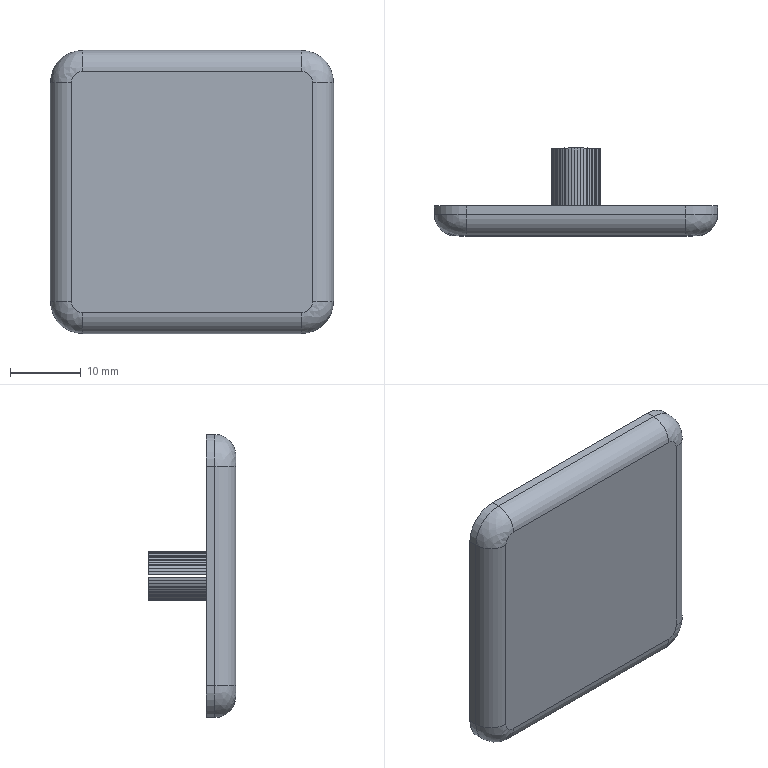Part | STEP file | End cap panel MK-EC-B-4040x4.2 | 1 solid | 127 faces | box 40 x 12.4 x 40 mm | volume 5038 mm3 | cylinder 62 | plane 61 | other 4 | commonest cylinder face diameters 6.6 x24 7 x23 9 x8 6 x4 4.9 x3